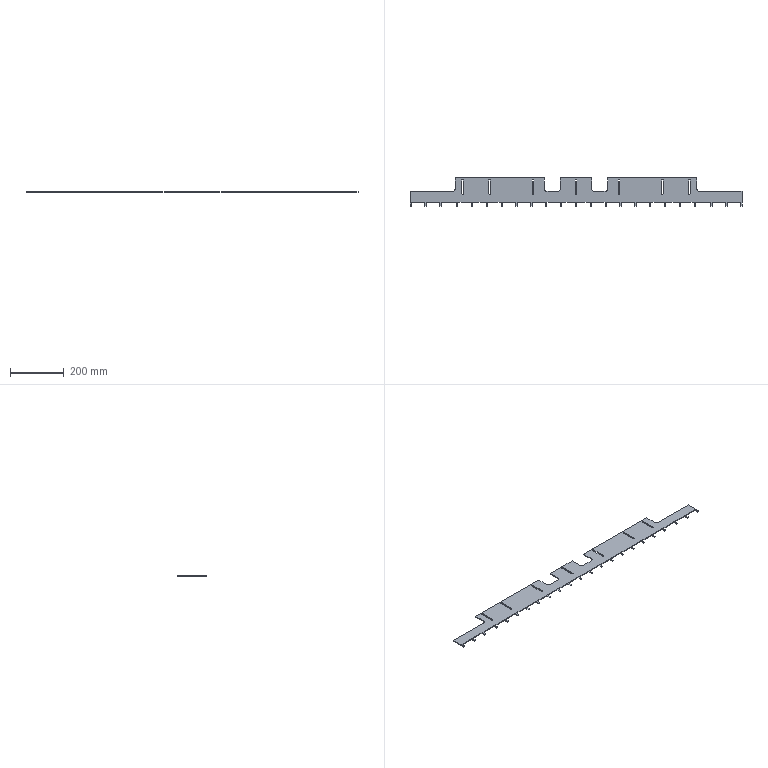Part | SolidWorks | features HoleWzd 2, ICE 2, MoveFace 2, Chamfer 1, Cut 1, Fillet 1, FlatPattern 1, LPattern 1, SMBaseFlange 1, SheetMetal 1 | 1 solid | 140 faces | box 1230 x 105 x 3 mm | volume 262856 mm3 | plane 120 | cylinder 20 | commonest cylinder face diameters 5.8 x14 20 x6